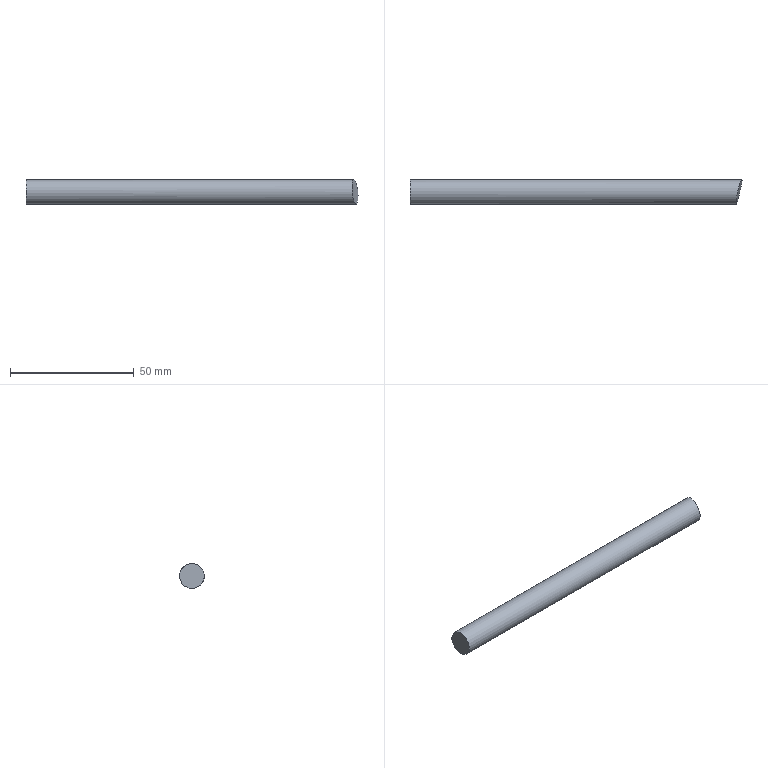Part | STEP file | solid 193 | 1 solid | 4 faces | box 134.268 x 10 x 10 mm | volume 10442 mm3 | spline 2 | cylinder 1 | plane 1 | commonest cylinder face diameters 10 x1